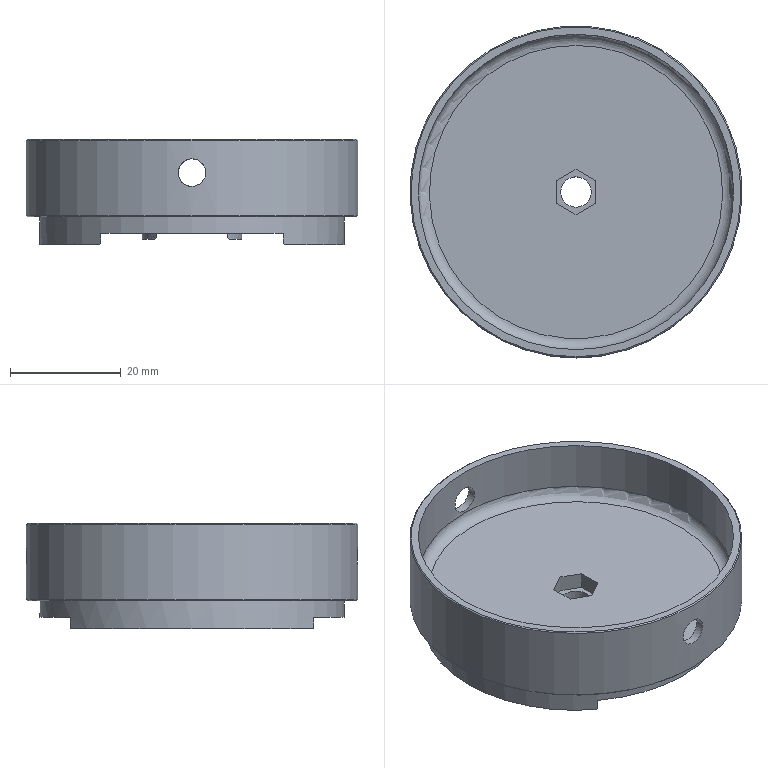Part | NX | 1 solid | 35 faces | box 60 x 60 x 19 mm | volume 19918 mm3 | plane 23 | cylinder 8 | cone 3 | torus 1 | commonest cylinder face diameters 5 x2 18 x2 5.5 x1 55 x1 57 x1 60 x1
STEP:
#1=CARTESIAN_POINT('',(0.,-2.75,-16.8));
#2=VERTEX_POINT('',#1);
#3=CARTESIAN_POINT('',(0.,0.,-16.8));
#4=DIRECTION('',(0.,0.,-1.));
#5=DIRECTION('',(0.,-1.,0.));
#6=AXIS2_PLACEMENT_3D('',#3,#4,#5);
#7=CIRCLE('',#6,2.75);
#8=EDGE_CURVE('',#2,#2,#7,.T.);
#9=ORIENTED_EDGE('',*,*,#8,.T.);
#10=EDGE_LOOP('',(#9));
#11=FACE_BOUND('',#10,.T.);
#12=CARTESIAN_POINT('',(0.,-2.75,-14.));
#13=VERTEX_POINT('',#12);
#14=CARTESIAN_POINT('',(0.,0.,-14.));
#15=DIRECTION('',(0.,0.,-1.));
#16=DIRECTION('',(0.,-1.,0.));
#17=AXIS2_PLACEMENT_3D('',#14,#15,#16);
#18=CIRCLE('',#17,2.75);
#19=EDGE_CURVE('',#13,#13,#18,.F.);
#20=ORIENTED_EDGE('',*,*,#19,.T.);
#21=EDGE_LOOP('',(#20));
#22=FACE_BOUND('',#21,.T.);
#23=CARTESIAN_POINT('',(0.,0.,0.));
#24=DIRECTION('',(0.,0.,-1.));
#25=DIRECTION('',(0.,-1.,0.));
#26=AXIS2_PLACEMENT_3D('',#23,#24,#25);
#27=CYLINDRICAL_SURFACE('',#26,2.75);
#28=ADVANCED_FACE('',(#11,#22),#27,.F.);
#29=CARTESIAN_POINT('',(-16.7,-21.849,-19.));
#30=VERTEX_POINT('',#29);
#31=CARTESIAN_POINT('',(-16.7,21.849,-19.));
#32=VERTEX_POINT('',#31);
#33=CARTESIAN_POINT('',(0.,0.,-19.));
#34=DIRECTION('',(0.,0.,-1.));
#35=DIRECTION('',(0.,-1.,0.));
#36=AXIS2_PLACEMENT_3D('',#33,#34,#35);
#37=CIRCLE('',#36,27.5);
#38=EDGE_CURVE('',#30,#32,#37,.T.);
#39=ORIENTED_EDGE('',*,*,#38,.T.);
#40=CARTESIAN_POINT('',(-16.7,-22.,-19.));
#41=DIRECTION('',(0.,-1.,0.));
#42=VECTOR('',#41,1000.);
#43=LINE('',#40,#42);
#44=EDGE_CURVE('',#32,#30,#43,.T.);
#45=ORIENTED_EDGE('',*,*,#44,.T.);
#46=EDGE_LOOP('',(#39,#45));
#47=FACE_BOUND('',#46,.T.);
#48=CARTESIAN_POINT('',(0.,0.,-19.));
#49=DIRECTION('',(0.,0.,-1.));
#50=DIRECTION('',(0.,-1.,0.));
#51=AXIS2_PLACEMENT_3D('',#48,#49,#50);
#52=PLANE('',#51);
#53=ADVANCED_FACE('',(#47),#52,.T.);
#54=CARTESIAN_POINT('',(0.,30.,-8.5));
#55=VERTEX_POINT('',#54);
#56=CARTESIAN_POINT('',(-1.961,29.948,-7.957));
#57=CARTESIAN_POINT('',(0.0004949,30.026,-8.771));
#58=CARTESIAN_POINT('',(1.959,29.948,-7.958));
#59=CARTESIAN_POINT('',(2.77,29.87,-6.002));
#60=CARTESIAN_POINT('',(1.96,29.948,-4.042));
#61=CARTESIAN_POINT('',(0.0004482,30.026,-3.23));
#62=CARTESIAN_POINT('',(-1.957,29.948,-4.039));
#63=CARTESIAN_POINT('',(-2.771,29.87,-5.997));
#64=CARTESIAN_POINT('',(-1.961,29.948,-7.957));
#65=CARTESIAN_POINT('',(0.0004949,30.026,-8.771));
#66=CARTESIAN_POINT('',(1.959,29.948,-7.958));
#67=B_SPLINE_CURVE_WITH_KNOTS('',3,(#56,#57,#58,#59,#60,#61,#62,#63,#64,#65,#66),.UNSPECIFIED.,.T.,.F.,(1,1,1,1,1,1,1,1,1,1,1,1,1,1,1),(-0.005864,-0.003909,-0.001955,0.,0.001955,0.003909,0.005864,0.007819,0.009773,0.01173,0.01368,0.01564,0.01759,0.01955,0.0215),.UNSPECIFIED.);
#68=EDGE_CURVE('',#55,#55,#67,.T.);
#69=ORIENTED_EDGE('',*,*,#68,.T.);
#70=EDGE_LOOP('',(#69));
#71=FACE_BOUND('',#70,.T.);
#72=CARTESIAN_POINT('',(-2.5,-29.896,-6.));
#73=VERTEX_POINT('',#72);
#74=CARTESIAN_POINT('',(-1.957,-29.948,-7.961));
#75=CARTESIAN_POINT('',(-2.771,-29.869,-6.));
#76=CARTESIAN_POINT('',(-1.958,-29.948,-4.041));
#77=CARTESIAN_POINT('',(-0.002118,-30.026,-3.23));
#78=CARTESIAN_POINT('',(1.958,-29.948,-4.04));
#79=CARTESIAN_POINT('',(2.77,-29.87,-6.));
#80=CARTESIAN_POINT('',(1.961,-29.948,-7.957));
#81=CARTESIAN_POINT('',(0.002777,-30.026,-8.771));
#82=CARTESIAN_POINT('',(-1.957,-29.948,-7.961));
#83=CARTESIAN_POINT('',(-2.771,-29.869,-6.));
#84=CARTESIAN_POINT('',(-1.958,-29.948,-4.041));
#85=B_SPLINE_CURVE_WITH_KNOTS('',3,(#74,#75,#76,#77,#78,#79,#80,#81,#82,#83,#84),.UNSPECIFIED.,.T.,.F.,(1,1,1,1,1,1,1,1,1,1,1,1,1,1,1),(-0.005864,-0.003909,-0.001955,0.,0.001955,0.003909,0.005864,0.007819,0.009773,0.01173,0.01368,0.01564,0.01759,0.01955,0.0215),.UNSPECIFIED.);
#86=EDGE_CURVE('',#73,#73,#85,.T.);
#87=ORIENTED_EDGE('',*,*,#86,.T.);
#88=EDGE_LOOP('',(#87));
#89=FACE_BOUND('',#88,.T.);
#90=CARTESIAN_POINT('',(0.,-30.,-13.8));
#91=VERTEX_POINT('',#90);
#92=CARTESIAN_POINT('',(0.,0.,-13.8));
#93=DIRECTION('',(0.,0.,-1.));
#94=DIRECTION('',(0.,-1.,0.));
#95=AXIS2_PLACEMENT_3D('',#92,#93,#94);
#96=CIRCLE('',#95,30.);
#97=EDGE_CURVE('',#91,#91,#96,.F.);
#98=ORIENTED_EDGE('',*,*,#97,.T.);
#99=EDGE_LOOP('',(#98));
#100=FACE_BOUND('',#99,.T.);
#101=CARTESIAN_POINT('',(0.,-30.,-0.2));
#102=VERTEX_POINT('',#101);
#103=CARTESIAN_POINT('',(0.,0.,-0.2));
#104=DIRECTION('',(0.,0.,-1.));
#105=DIRECTION('',(0.,-1.,0.));
#106=AXIS2_PLACEMENT_3D('',#103,#104,#105);
#107=CIRCLE('',#106,30.);
#108=EDGE_CURVE('',#102,#102,#107,.T.);
#109=ORIENTED_EDGE('',*,*,#108,.T.);
#110=EDGE_LOOP('',(#109));
#111=FACE_BOUND('',#110,.T.);
#112=CARTESIAN_POINT('',(0.,0.,-19.));
#113=DIRECTION('',(0.,0.,1.));
#114=DIRECTION('',(0.,1.,0.));
#115=AXIS2_PLACEMENT_3D('',#112,#113,#114);
#116=CYLINDRICAL_SURFACE('',#115,30.);
#117=ADVANCED_FACE('',(#71,#89,#100,#111),#116,.T.);
#118=CARTESIAN_POINT('',(0.,-29.8,0.));
#119=VERTEX_POINT('',#118);
#120=CARTESIAN_POINT('',(0.,0.,0.));
#121=DIRECTION('',(0.,0.,-1.));
#122=DIRECTION('',(0.,-1.,0.));
#123=AXIS2_PLACEMENT_3D('',#120,#121,#122);
#124=CIRCLE('',#123,29.8);
#125=EDGE_CURVE('',#119,#119,#124,.F.);
#126=ORIENTED_EDGE('',*,*,#125,.T.);
#127=EDGE_LOOP('',(#126));
#128=FACE_BOUND('',#127,.T.);
#129=CARTESIAN_POINT('',(0.,28.5,0.));
#130=VERTEX_POINT('',#129);
#131=CARTESIAN_POINT('',(0.,0.,0.));
#132=DIRECTION('',(0.,0.,1.));
#133=DIRECTION('',(0.,1.,0.));
#134=AXIS2_PLACEMENT_3D('',#131,#132,#133);
#135=CIRCLE('',#134,28.5);
#136=EDGE_CURVE('',#130,#130,#135,.T.);
#137=ORIENTED_EDGE('',*,*,#136,.F.);
#138=EDGE_LOOP('',(#137));
#139=FACE_BOUND('',#138,.T.);
#140=CARTESIAN_POINT('',(0.,0.,0.));
#141=DIRECTION('',(0.,0.,-1.));
#142=DIRECTION('',(0.,-1.,0.));
#143=AXIS2_PLACEMENT_3D('',#140,#141,#142);
#144=PLANE('',#143);
#145=ADVANCED_FACE('',(#128,#139),#144,.F.);
#146=CARTESIAN_POINT('',(0.,-29.8,-14.));
#147=VERTEX_POINT('',#146);
#148=CARTESIAN_POINT('',(0.,0.,-14.));
#149=DIRECTION('',(0.,0.,-1.));
#150=DIRECTION('',(0.,-1.,0.));
#151=AXIS2_PLACEMENT_3D('',#148,#149,#150);
#152=CIRCLE('',#151,29.8);
#153=EDGE_CURVE('',#147,#147,#152,.T.);
#154=ORIENTED_EDGE('',*,*,#153,.T.);
#155=EDGE_LOOP('',(#154));
#156=FACE_BOUND('',#155,.T.);
#157=CARTESIAN_POINT('',(0.,-27.5,-14.));
#158=VERTEX_POINT('',#157);
#159=CARTESIAN_POINT('',(0.,0.,-14.));
#160=DIRECTION('',(0.,0.,-1.));
#161=DIRECTION('',(0.,-1.,0.));
#162=AXIS2_PLACEMENT_3D('',#159,#160,#161);
#163=CIRCLE('',#162,27.5);
#164=EDGE_CURVE('',#158,#158,#163,.T.);
#165=ORIENTED_EDGE('',*,*,#164,.F.);
#166=EDGE_LOOP('',(#165));
#167=FACE_BOUND('',#166,.T.);
#168=CARTESIAN_POINT('',(0.,0.,-14.));
#169=DIRECTION('',(0.,0.,-1.));
#170=DIRECTION('',(0.,-1.,0.));
#171=AXIS2_PLACEMENT_3D('',#168,#169,#170);
#172=PLANE('',#171);
#173=ADVANCED_FACE('',(#156,#167),#172,.T.);
#174=CARTESIAN_POINT('',(-16.5,22.,-18.8));
#175=VERTEX_POINT('',#174);
#176=CARTESIAN_POINT('',(-16.5,22.,-17.));
#177=VERTEX_POINT('',#176);
#178=CARTESIAN_POINT('',(-16.5,22.,-17.));
#179=DIRECTION('',(0.,0.,-1.));
#180=VECTOR('',#179,1000.);
#181=LINE('',#178,#180);
#182=EDGE_CURVE('',#175,#177,#181,.F.);
#183=ORIENTED_EDGE('',*,*,#182,.F.);
#184=CARTESIAN_POINT('',(0.,0.,-2.3));
#185=DIRECTION('',(0.7071,0.,-0.7071));
#186=DIRECTION('',(-0.7071,0.,-0.7071));
#187=AXIS2_PLACEMENT_3D('',#184,#185,#186);
#188=ELLIPSE('',#187,38.891,27.5);
#189=EDGE_CURVE('',#175,#32,#188,.F.);
#190=ORIENTED_EDGE('',*,*,#189,.T.);
#191=ORIENTED_EDGE('',*,*,#38,.F.);
#192=CARTESIAN_POINT('',(-16.5,-22.,-18.8));
#193=VERTEX_POINT('',#192);
#194=CARTESIAN_POINT('',(0.,0.,-2.3));
#195=DIRECTION('',(0.7071,0.,-0.7071));
#196=DIRECTION('',(-0.7071,0.,-0.7071));
#197=AXIS2_PLACEMENT_3D('',#194,#195,#196);
#198=ELLIPSE('',#197,38.891,27.5);
#199=EDGE_CURVE('',#30,#193,#198,.F.);
#200=ORIENTED_EDGE('',*,*,#199,.T.);
#201=CARTESIAN_POINT('',(-16.5,-22.,-17.));
#202=VERTEX_POINT('',#201);
#203=CARTESIAN_POINT('',(-16.5,-22.,-17.));
#204=DIRECTION('',(0.,0.,-1.));
#205=VECTOR('',#204,1000.);
#206=LINE('',#203,#205);
#207=EDGE_CURVE('',#193,#202,#206,.F.);
#208=ORIENTED_EDGE('',*,*,#207,.T.);
#209=CARTESIAN_POINT('',(16.5,-22.,-17.));
#210=VERTEX_POINT('',#209);
#211=CARTESIAN_POINT('',(0.,0.,-17.));
#212=DIRECTION('',(0.,0.,-1.));
#213=DIRECTION('',(0.,-1.,0.));
#214=AXIS2_PLACEMENT_3D('',#211,#212,#213);
#215=CIRCLE('',#214,27.5);
#216=EDGE_CURVE('',#210,#202,#215,.T.);
#217=ORIENTED_EDGE('',*,*,#216,.F.);
#218=CARTESIAN_POINT('',(16.5,-22.,-18.8));
#219=VERTEX_POINT('',#218);
#220=CARTESIAN_POINT('',(16.5,-22.,-17.));
#221=DIRECTION('',(0.,0.,-1.));
#222=VECTOR('',#221,1000.);
#223=LINE('',#220,#222);
#224=EDGE_CURVE('',#219,#210,#223,.F.);
#225=ORIENTED_EDGE('',*,*,#224,.F.);
#226=CARTESIAN_POINT('',(16.7,-21.849,-19.));
#227=VERTEX_POINT('',#226);
#228=CARTESIAN_POINT('',(0.,0.,-2.3));
#229=DIRECTION('',(-0.7071,0.,-0.7071));
#230=DIRECTION('',(0.7071,0.,-0.7071));
#231=AXIS2_PLACEMENT_3D('',#228,#229,#230);
#232=ELLIPSE('',#231,38.891,27.5);
#233=EDGE_CURVE('',#219,#227,#232,.F.);
#234=ORIENTED_EDGE('',*,*,#233,.T.);
#235=CARTESIAN_POINT('',(16.7,21.849,-19.));
#236=VERTEX_POINT('',#235);
#237=CARTESIAN_POINT('',(0.,0.,-19.));
#238=DIRECTION('',(0.,0.,-1.));
#239=DIRECTION('',(0.,-1.,0.));
#240=AXIS2_PLACEMENT_3D('',#237,#238,#239);
#241=CIRCLE('',#240,27.5);
#242=EDGE_CURVE('',#236,#227,#241,.T.);
#243=ORIENTED_EDGE('',*,*,#242,.F.);
#244=CARTESIAN_POINT('',(16.5,22.,-18.8));
#245=VERTEX_POINT('',#244);
#246=CARTESIAN_POINT('',(0.,0.,-2.3));
#247=DIRECTION('',(-0.7071,0.,-0.7071));
#248=DIRECTION('',(0.7071,0.,-0.7071));
#249=AXIS2_PLACEMENT_3D('',#246,#247,#248);
#250=ELLIPSE('',#249,38.891,27.5);
#251=EDGE_CURVE('',#236,#245,#250,.F.);
#252=ORIENTED_EDGE('',*,*,#251,.T.);
#253=CARTESIAN_POINT('',(16.5,22.,-17.));
#254=VERTEX_POINT('',#253);
#255=CARTESIAN_POINT('',(16.5,22.,-17.));
#256=DIRECTION('',(0.,0.,-1.));
#257=VECTOR('',#256,1000.);
#258=LINE('',#255,#257);
#259=EDGE_CURVE('',#245,#254,#258,.F.);
#260=ORIENTED_EDGE('',*,*,#259,.T.);
#261=CARTESIAN_POINT('',(0.,0.,-17.));
#262=DIRECTION('',(0.,0.,-1.));
#263=DIRECTION('',(0.,-1.,0.));
#264=AXIS2_PLACEMENT_3D('',#261,#262,#263);
#265=CIRCLE('',#264,27.5);
#266=EDGE_CURVE('',#177,#254,#265,.T.);
#267=ORIENTED_EDGE('',*,*,#266,.F.);
#268=EDGE_LOOP('',(#183,#190,#191,#200,#208,#217,#225,#234,#243,#252,#260,#267));
#269=FACE_BOUND('',#268,.T.);
#270=ORIENTED_EDGE('',*,*,#164,.T.);
#271=EDGE_LOOP('',(#270));
#272=FACE_BOUND('',#271,.T.);
#273=CARTESIAN_POINT('',(0.,0.,-14.));
#274=DIRECTION('',(0.,0.,-1.));
#275=DIRECTION('',(0.,-1.,0.));
#276=AXIS2_PLACEMENT_3D('',#273,#274,#275);
#277=CYLINDRICAL_SURFACE('',#276,27.5);
#278=ADVANCED_FACE('',(#269,#272),#277,.T.);
#279=ORIENTED_EDGE('',*,*,#242,.T.);
#280=CARTESIAN_POINT('',(16.7,22.,-19.));
#281=DIRECTION('',(0.,1.,0.));
#282=VECTOR('',#281,1000.);
#283=LINE('',#280,#282);
#284=EDGE_CURVE('',#227,#236,#283,.T.);
#285=ORIENTED_EDGE('',*,*,#284,.T.);
#286=EDGE_LOOP('',(#279,#285));
#287=FACE_BOUND('',#286,.T.);
#288=CARTESIAN_POINT('',(0.,0.,-19.));
#289=DIRECTION('',(0.,0.,-1.));
#290=DIRECTION('',(0.,-1.,0.));
#291=AXIS2_PLACEMENT_3D('',#288,#289,#290);
#292=PLANE('',#291);
#293=ADVANCED_FACE('',(#287),#292,.T.);
#294=ORIENTED_EDGE('',*,*,#207,.F.);
#295=CARTESIAN_POINT('',(-16.5,22.,-18.8));
#296=DIRECTION('',(0.,1.,0.));
#297=VECTOR('',#296,1000.);
#298=LINE('',#295,#297);
#299=EDGE_CURVE('',#193,#175,#298,.T.);
#300=ORIENTED_EDGE('',*,*,#299,.T.);
#301=ORIENTED_EDGE('',*,*,#182,.T.);
#302=CARTESIAN_POINT('',(-16.5,22.,-17.));
#303=DIRECTION('',(0.,1.,0.));
#304=VECTOR('',#303,1000.);
#305=LINE('',#302,#304);
#306=EDGE_CURVE('',#202,#177,#305,.T.);
#307=ORIENTED_EDGE('',*,*,#306,.F.);
#308=EDGE_LOOP('',(#294,#300,#301,#307));
#309=FACE_BOUND('',#308,.T.);
#310=CARTESIAN_POINT('',(-16.5,22.,-17.));
#311=DIRECTION('',(-1.,0.,0.));
#312=DIRECTION('',(0.,1.,0.));
#313=AXIS2_PLACEMENT_3D('',#310,#311,#312);
#314=PLANE('',#313);
#315=ADVANCED_FACE('',(#309),#314,.F.);
#316=ORIENTED_EDGE('',*,*,#259,.F.);
#317=CARTESIAN_POINT('',(16.5,-22.,-18.8));
#318=DIRECTION('',(0.,-1.,0.));
#319=VECTOR('',#318,1000.);
#320=LINE('',#317,#319);
#321=EDGE_CURVE('',#245,#219,#320,.T.);
#322=ORIENTED_EDGE('',*,*,#321,.T.);
#323=ORIENTED_EDGE('',*,*,#224,.T.);
#324=CARTESIAN_POINT('',(16.5,22.,-17.));
#325=DIRECTION('',(0.,-1.,0.));
#326=VECTOR('',#325,1000.);
#327=LINE('',#324,#326);
#328=EDGE_CURVE('',#254,#210,#327,.T.);
#329=ORIENTED_EDGE('',*,*,#328,.F.);
#330=EDGE_LOOP('',(#316,#322,#323,#329));
#331=FACE_BOUND('',#330,.T.);
#332=CARTESIAN_POINT('',(16.5,22.,-17.));
#333=DIRECTION('',(1.,0.,0.));
#334=DIRECTION('',(0.,-1.,0.));
#335=AXIS2_PLACEMENT_3D('',#332,#333,#334);
#336=PLANE('',#335);
#337=ADVANCED_FACE('',(#331),#336,.F.);
#338=CARTESIAN_POINT('',(0.,-2.95,-17.));
#339=VERTEX_POINT('',#338);
#340=CARTESIAN_POINT('',(0.,0.,-17.));
#341=DIRECTION('',(0.,0.,-1.));
#342=DIRECTION('',(0.,-1.,0.));
#343=AXIS2_PLACEMENT_3D('',#340,#341,#342);
#344=CIRCLE('',#343,2.95);
#345=EDGE_CURVE('',#339,#339,#344,.F.);
#346=ORIENTED_EDGE('',*,*,#345,.T.);
#347=EDGE_LOOP('',(#346));
#348=FACE_BOUND('',#347,.T.);
#349=CARTESIAN_POINT('',(-6.5,6.225,-17.));
#350=VERTEX_POINT('',#349);
#351=CARTESIAN_POINT('',(-6.5,-6.225,-17.));
#352=VERTEX_POINT('',#351);
#353=CARTESIAN_POINT('',(-6.5,6.225,-17.));
#354=DIRECTION('',(0.,-1.,0.));
#355=VECTOR('',#354,1000.);
#356=LINE('',#353,#355);
#357=EDGE_CURVE('',#350,#352,#356,.T.);
#358=ORIENTED_EDGE('',*,*,#357,.F.);
#359=CARTESIAN_POINT('',(0.,0.,-17.));
#360=DIRECTION('',(0.,0.,-1.));
#361=DIRECTION('',(0.,-1.,0.));
#362=AXIS2_PLACEMENT_3D('',#359,#360,#361);
#363=CIRCLE('',#362,9.);
#364=EDGE_CURVE('',#352,#350,#363,.T.);
#365=ORIENTED_EDGE('',*,*,#364,.F.);
#366=EDGE_LOOP('',(#358,#365));
#367=FACE_BOUND('',#366,.T.);
#368=CARTESIAN_POINT('',(6.5,-6.225,-17.));
#369=VERTEX_POINT('',#368);
#370=CARTESIAN_POINT('',(6.5,6.225,-17.));
#371=VERTEX_POINT('',#370);
#372=CARTESIAN_POINT('',(6.5,6.225,-17.));
#373=DIRECTION('',(0.,1.,0.));
#374=VECTOR('',#373,1000.);
#375=LINE('',#372,#374);
#376=EDGE_CURVE('',#369,#371,#375,.T.);
#377=ORIENTED_EDGE('',*,*,#376,.F.);
#378=CARTESIAN_POINT('',(0.,0.,-17.));
#379=DIRECTION('',(0.,0.,-1.));
#380=DIRECTION('',(0.,-1.,0.));
#381=AXIS2_PLACEMENT_3D('',#378,#379,#380);
#382=CIRCLE('',#381,9.);
#383=EDGE_CURVE('',#371,#369,#382,.T.);
#384=ORIENTED_EDGE('',*,*,#383,.F.);
#385=EDGE_LOOP('',(#377,#384));
#386=FACE_BOUND('',#385,.T.);
#387=ORIENTED_EDGE('',*,*,#266,.T.);
#388=ORIENTED_EDGE('',*,*,#328,.T.);
#389=ORIENTED_EDGE('',*,*,#216,.T.);
#390=ORIENTED_EDGE('',*,*,#306,.T.);
#391=EDGE_LOOP('',(#387,#388,#389,#390));
#392=FACE_BOUND('',#391,.T.);
#393=CARTESIAN_POINT('',(0.,0.,-17.));
#394=DIRECTION('',(0.,0.,-1.));
#395=DIRECTION('',(0.,-1.,0.));
#396=AXIS2_PLACEMENT_3D('',#393,#394,#395);
#397=PLANE('',#396);
#398=ADVANCED_FACE('',(#348,#367,#386,#392),#397,.T.);
#399=CARTESIAN_POINT('',(6.7,6.009,-18.));
#400=VERTEX_POINT('',#399);
#401=CARTESIAN_POINT('',(6.7,-6.009,-18.));
#402=VERTEX_POINT('',#401);
#403=CARTESIAN_POINT('',(0.,0.,-18.));
#404=DIRECTION('',(0.,0.,1.));
#405=DIRECTION('',(0.,1.,0.));
#406=AXIS2_PLACEMENT_3D('',#403,#404,#405);
#407=CIRCLE('',#406,9.);
#408=EDGE_CURVE('',#400,#402,#407,.F.);
#409=ORIENTED_EDGE('',*,*,#408,.F.);
#410=CARTESIAN_POINT('',(6.5,6.225,-17.8));
#411=VERTEX_POINT('',#410);
#412=CARTESIAN_POINT('',(0.,0.,-11.3));
#413=DIRECTION('',(-0.7071,0.,-0.7071));
#414=DIRECTION('',(0.7071,0.,-0.7071));
#415=AXIS2_PLACEMENT_3D('',#412,#413,#414);
#416=ELLIPSE('',#415,12.728,9.);
#417=EDGE_CURVE('',#400,#411,#416,.F.);
#418=ORIENTED_EDGE('',*,*,#417,.T.);
#419=CARTESIAN_POINT('',(6.5,6.225,-17.));
#420=DIRECTION('',(0.,0.,-1.));
#421=VECTOR('',#420,1000.);
#422=LINE('',#419,#421);
#423=EDGE_CURVE('',#411,#371,#422,.F.);
#424=ORIENTED_EDGE('',*,*,#423,.T.);
#425=ORIENTED_EDGE('',*,*,#383,.T.);
#426=CARTESIAN_POINT('',(6.5,-6.225,-17.8));
#427=VERTEX_POINT('',#426);
#428=CARTESIAN_POINT('',(6.5,-6.225,-17.));
#429=DIRECTION('',(0.,0.,-1.));
#430=VECTOR('',#429,1000.);
#431=LINE('',#428,#430);
#432=EDGE_CURVE('',#427,#369,#431,.F.);
#433=ORIENTED_EDGE('',*,*,#432,.F.);
#434=CARTESIAN_POINT('',(0.,0.,-11.3));
#435=DIRECTION('',(-0.7071,0.,-0.7071));
#436=DIRECTION('',(0.7071,0.,-0.7071));
#437=AXIS2_PLACEMENT_3D('',#434,#435,#436);
#438=ELLIPSE('',#437,12.728,9.);
#439=EDGE_CURVE('',#427,#402,#438,.F.);
#440=ORIENTED_EDGE('',*,*,#439,.T.);
#441=EDGE_LOOP('',(#409,#418,#424,#425,#433,#440));
#442=FACE_BOUND('',#441,.T.);
#443=CARTESIAN_POINT('',(0.,0.,-17.));
#444=DIRECTION('',(0.,0.,-1.));
#445=DIRECTION('',(0.,-1.,0.));
#446=AXIS2_PLACEMENT_3D('',#443,#444,#445);
#447=CYLINDRICAL_SURFACE('',#446,9.);
#448=ADVANCED_FACE('',(#442),#447,.T.);
#449=ORIENTED_EDGE('',*,*,#423,.F.);
#450=CARTESIAN_POINT('',(6.5,-6.225,-17.8));
#451=DIRECTION('',(0.,-1.,0.));
#452=VECTOR('',#451,1000.);
#453=LINE('',#450,#452);
#454=EDGE_CURVE('',#411,#427,#453,.T.);
#455=ORIENTED_EDGE('',*,*,#454,.T.);
#456=ORIENTED_EDGE('',*,*,#432,.T.);
#457=ORIENTED_EDGE('',*,*,#376,.T.);
#458=EDGE_LOOP('',(#449,#455,#456,#457));
#459=FACE_BOUND('',#458,.T.);
#460=CARTESIAN_POINT('',(6.5,6.225,-17.));
#461=DIRECTION('',(-1.,0.,0.));
#462=DIRECTION('',(0.,1.,0.));
#463=AXIS2_PLACEMENT_3D('',#460,#461,#462);
#464=PLANE('',#463);
#465=ADVANCED_FACE('',(#459),#464,.T.);
#466=CARTESIAN_POINT('',(-6.7,-6.009,-18.));
#467=VERTEX_POINT('',#466);
#468=CARTESIAN_POINT('',(-6.7,6.009,-18.));
#469=VERTEX_POINT('',#468);
#470=CARTESIAN_POINT('',(0.,0.,-18.));
#471=DIRECTION('',(0.,0.,1.));
#472=DIRECTION('',(0.,1.,0.));
#473=AXIS2_PLACEMENT_3D('',#470,#471,#472);
#474=CIRCLE('',#473,9.);
#475=EDGE_CURVE('',#467,#469,#474,.F.);
#476=ORIENTED_EDGE('',*,*,#475,.F.);
#477=CARTESIAN_POINT('',(-6.5,-6.225,-17.8));
#478=VERTEX_POINT('',#477);
#479=CARTESIAN_POINT('',(0.,0.,-11.3));
#480=DIRECTION('',(0.7071,0.,-0.7071));
#481=DIRECTION('',(-0.7071,0.,-0.7071));
#482=AXIS2_PLACEMENT_3D('',#479,#480,#481);
#483=ELLIPSE('',#482,12.728,9.);
#484=EDGE_CURVE('',#467,#478,#483,.F.);
#485=ORIENTED_EDGE('',*,*,#484,.T.);
#486=CARTESIAN_POINT('',(-6.5,-6.225,-17.));
#487=DIRECTION('',(0.,0.,-1.));
#488=VECTOR('',#487,1000.);
#489=LINE('',#486,#488);
#490=EDGE_CURVE('',#478,#352,#489,.F.);
#491=ORIENTED_EDGE('',*,*,#490,.T.);
#492=ORIENTED_EDGE('',*,*,#364,.T.);
#493=CARTESIAN_POINT('',(-6.5,6.225,-17.8));
#494=VERTEX_POINT('',#493);
#495=CARTESIAN_POINT('',(-6.5,6.225,-17.));
#496=DIRECTION('',(0.,0.,-1.));
#497=VECTOR('',#496,1000.);
#498=LINE('',#495,#497);
#499=EDGE_CURVE('',#494,#350,#498,.F.);
#500=ORIENTED_EDGE('',*,*,#499,.F.);
#501=CARTESIAN_POINT('',(0.,0.,-11.3));
#502=DIRECTION('',(0.7071,0.,-0.7071));
#503=DIRECTION('',(-0.7071,0.,-0.7071));
#504=AXIS2_PLACEMENT_3D('',#501,#502,#503);
#505=ELLIPSE('',#504,12.728,9.);
#506=EDGE_CURVE('',#494,#469,#505,.F.);
#507=ORIENTED_EDGE('',*,*,#506,.T.);
#508=EDGE_LOOP('',(#476,#485,#491,#492,#500,#507));
#509=FACE_BOUND('',#508,.T.);
#510=CARTESIAN_POINT('',(0.,0.,-17.));
#511=DIRECTION('',(0.,0.,-1.));
#512=DIRECTION('',(0.,-1.,0.));
#513=AXIS2_PLACEMENT_3D('',#510,#511,#512);
#514=CYLINDRICAL_SURFACE('',#513,9.);
#515=ADVANCED_FACE('',(#509),#514,.T.);
#516=ORIENTED_EDGE('',*,*,#490,.F.);
#517=CARTESIAN_POINT('',(-6.5,6.225,-17.8));
#518=DIRECTION('',(0.,1.,0.));
#519=VECTOR('',#518,1000.);
#520=LINE('',#517,#519);
#521=EDGE_CURVE('',#478,#494,#520,.T.);
#522=ORIENTED_EDGE('',*,*,#521,.T.);
#523=ORIENTED_EDGE('',*,*,#499,.T.);
#524=ORIENTED_EDGE('',*,*,#357,.T.);
#525=EDGE_LOOP('',(#516,#522,#523,#524));
#526=FACE_BOUND('',#525,.T.);
#527=CARTESIAN_POINT('',(-6.5,6.225,-17.));
#528=DIRECTION('',(1.,0.,0.));
#529=DIRECTION('',(0.,-1.,0.));
#530=AXIS2_PLACEMENT_3D('',#527,#528,#529);
#531=PLANE('',#530);
#532=ADVANCED_FACE('',(#526),#531,.T.);
#533=CARTESIAN_POINT('',(0.,26.5,-11.));
#534=VERTEX_POINT('',#533);
#535=CARTESIAN_POINT('',(0.,0.,-11.));
#536=DIRECTION('',(0.,0.,1.));
#537=DIRECTION('',(0.,1.,0.));
#538=AXIS2_PLACEMENT_3D('',#535,#536,#537);
#539=CIRCLE('',#538,26.5);
#540=EDGE_CURVE('',#534,#534,#539,.T.);
#541=ORIENTED_EDGE('',*,*,#540,.T.);
#542=EDGE_LOOP('',(#541));
#543=FACE_BOUND('',#542,.T.);
#544=CARTESIAN_POINT('',(0.,-4.099,-11.));
#545=VERTEX_POINT('',#544);
#546=CARTESIAN_POINT('',(3.55,-2.05,-11.));
#547=VERTEX_POINT('',#546);
#548=CARTESIAN_POINT('',(0.,-4.099,-11.));
#549=DIRECTION('',(0.866,0.5,0.));
#550=VECTOR('',#549,1000.);
#551=LINE('',#548,#550);
#552=EDGE_CURVE('',#545,#547,#551,.T.);
#553=ORIENTED_EDGE('',*,*,#552,.F.);
#554=CARTESIAN_POINT('',(-3.55,-2.05,-11.));
#555=VERTEX_POINT('',#554);
#556=CARTESIAN_POINT('',(-3.55,-2.05,-11.));
#557=DIRECTION('',(0.866,-0.5,0.));
#558=VECTOR('',#557,1000.);
#559=LINE('',#556,#558);
#560=EDGE_CURVE('',#555,#545,#559,.T.);
#561=ORIENTED_EDGE('',*,*,#560,.F.);
#562=CARTESIAN_POINT('',(-3.55,2.05,-11.));
#563=VERTEX_POINT('',#562);
#564=CARTESIAN_POINT('',(-3.55,2.05,-11.));
#565=DIRECTION('',(0.,-1.,0.));
#566=VECTOR('',#565,1000.);
#567=LINE('',#564,#566);
#568=EDGE_CURVE('',#563,#555,#567,.T.);
#569=ORIENTED_EDGE('',*,*,#568,.F.);
#570=CARTESIAN_POINT('',(0.,4.099,-11.));
#571=VERTEX_POINT('',#570);
#572=CARTESIAN_POINT('',(0.,4.099,-11.));
#573=DIRECTION('',(-0.866,-0.5,0.));
#574=VECTOR('',#573,1000.);
#575=LINE('',#572,#574);
#576=EDGE_CURVE('',#571,#563,#575,.T.);
#577=ORIENTED_EDGE('',*,*,#576,.F.);
#578=CARTESIAN_POINT('',(3.55,2.05,-11.));
#579=VERTEX_POINT('',#578);
#580=CARTESIAN_POINT('',(3.55,2.05,-11.));
#581=DIRECTION('',(-0.866,0.5,0.));
#582=VECTOR('',#581,1000.);
#583=LINE('',#580,#582);
#584=EDGE_CURVE('',#579,#571,#583,.T.);
#585=ORIENTED_EDGE('',*,*,#584,.F.);
#586=CARTESIAN_POINT('',(3.55,-2.05,-11.));
#587=DIRECTION('',(0.,1.,0.));
#588=VECTOR('',#587,1000.);
#589=LINE('',#586,#588);
#590=EDGE_CURVE('',#547,#579,#589,.T.);
#591=ORIENTED_EDGE('',*,*,#590,.F.);
#592=EDGE_LOOP('',(#553,#561,#569,#577,#585,#591));
#593=FACE_BOUND('',#592,.T.);
#594=CARTESIAN_POINT('',(0.,0.,-11.));
#595=DIRECTION('',(0.,0.,1.));
#596=DIRECTION('',(0.,1.,0.));
#597=AXIS2_PLACEMENT_3D('',#594,#595,#596);
#598=PLANE('',#597);
#599=ADVANCED_FACE('',(#543,#593),#598,.T.);
#600=CARTESIAN_POINT('',(0.,28.5,-8.5));
#601=VERTEX_POINT('',#600);
#602=CARTESIAN_POINT('',(1.961,28.445,-7.957));
#603=CARTESIAN_POINT('',(-0.0004939,28.527,-8.771));
#604=CARTESIAN_POINT('',(-1.959,28.445,-7.958));
#605=CARTESIAN_POINT('',(-2.77,28.363,-6.002));
#606=CARTESIAN_POINT('',(-1.96,28.445,-4.042));
#607=CARTESIAN_POINT('',(-0.0004583,28.527,-3.23));
#608=CARTESIAN_POINT('',(1.957,28.445,-4.039));
#609=CARTESIAN_POINT('',(2.771,28.363,-5.997));
#610=CARTESIAN_POINT('',(1.961,28.445,-7.957));
#611=CARTESIAN_POINT('',(-0.0004939,28.527,-8.771));
#612=CARTESIAN_POINT('',(-1.959,28.445,-7.958));
#613=B_SPLINE_CURVE_WITH_KNOTS('',3,(#602,#603,#604,#605,#606,#607,#608,#609,#610,#611,#612),.UNSPECIFIED.,.T.,.F.,(1,1,1,1,1,1,1,1,1,1,1,1,1,1,1),(-0.005864,-0.003909,-0.001955,0.,0.001955,0.003909,0.005864,0.007819,0.009774,0.01173,0.01368,0.01564,0.01759,0.01955,0.0215),.UNSPECIFIED.);
#614=EDGE_CURVE('',#601,#601,#613,.T.);
#615=ORIENTED_EDGE('',*,*,#614,.T.);
#616=EDGE_LOOP('',(#615));
#617=FACE_BOUND('',#616,.T.);
#618=CARTESIAN_POINT('',(-2.5,-28.39,-6.));
#619=VERTEX_POINT('',#618);
#620=CARTESIAN_POINT('',(-1.957,-28.445,-4.039));
#621=CARTESIAN_POINT('',(-2.771,-28.363,-6.));
#622=CARTESIAN_POINT('',(-1.958,-28.445,-7.959));
#623=CARTESIAN_POINT('',(-0.002129,-28.527,-8.77));
#624=CARTESIAN_POINT('',(1.958,-28.445,-7.96));
#625=CARTESIAN_POINT('',(2.77,-28.363,-6.));
#626=CARTESIAN_POINT('',(1.961,-28.445,-4.043));
#627=CARTESIAN_POINT('',(0.002754,-28.527,-3.229));
#628=CARTESIAN_POINT('',(-1.957,-28.445,-4.039));
#629=CARTESIAN_POINT('',(-2.771,-28.363,-6.));
#630=CARTESIAN_POINT('',(-1.958,-28.445,-7.959));
#631=B_SPLINE_CURVE_WITH_KNOTS('',3,(#620,#621,#622,#623,#624,#625,#626,#627,#628,#629,#630),.UNSPECIFIED.,.T.,.F.,(1,1,1,1,1,1,1,1,1,1,1,1,1,1,1),(-0.005864,-0.003909,-0.001955,0.,0.001955,0.003909,0.005864,0.007819,0.009774,0.01173,0.01368,0.01564,0.01759,0.01955,0.0215),.UNSPECIFIED.);
#632=EDGE_CURVE('',#619,#619,#631,.T.);
#633=ORIENTED_EDGE('',*,*,#632,.T.);
#634=EDGE_LOOP('',(#633));
#635=FACE_BOUND('',#634,.T.);
#636=CARTESIAN_POINT('',(0.,28.5,-9.));
#637=VERTEX_POINT('',#636);
#638=CARTESIAN_POINT('',(0.,0.,-9.));
#639=DIRECTION('',(0.,0.,1.));
#640=DIRECTION('',(0.,1.,0.));
#641=AXIS2_PLACEMENT_3D('',#638,#639,#640);
#642=CIRCLE('',#641,28.5);
#643=EDGE_CURVE('',#637,#637,#642,.F.);
#644=ORIENTED_EDGE('',*,*,#643,.T.);
#645=EDGE_LOOP('',(#644));
#646=FACE_BOUND('',#645,.T.);
#647=ORIENTED_EDGE('',*,*,#136,.T.);
#648=EDGE_LOOP('',(#647));
#649=FACE_BOUND('',#648,.T.);
#650=CARTESIAN_POINT('',(0.,0.,-11.));
#651=DIRECTION('',(0.,0.,1.));
#652=DIRECTION('',(0.,1.,0.));
#653=AXIS2_PLACEMENT_3D('',#650,#651,#652);
#654=CYLINDRICAL_SURFACE('',#653,28.5);
#655=ADVANCED_FACE('',(#617,#635,#646,#649),#654,.F.);
#656=CARTESIAN_POINT('',(-3.55,-2.05,-14.));
#657=VERTEX_POINT('',#656);
#658=CARTESIAN_POINT('',(0.,-4.099,-14.));
#659=VERTEX_POINT('',#658);
#660=CARTESIAN_POINT('',(-3.55,-2.05,-14.));
#661=DIRECTION('',(0.866,-0.5,0.));
#662=VECTOR('',#661,1000.);
#663=LINE('',#660,#662);
#664=EDGE_CURVE('',#657,#659,#663,.T.);
#665=ORIENTED_EDGE('',*,*,#664,.T.);
#666=CARTESIAN_POINT('',(3.55,-2.05,-14.));
#667=VERTEX_POINT('',#666);
#668=CARTESIAN_POINT('',(0.,-4.099,-14.));
#669=DIRECTION('',(0.866,0.5,0.));
#670=VECTOR('',#669,1000.);
#671=LINE('',#668,#670);
#672=EDGE_CURVE('',#659,#667,#671,.T.);
#673=ORIENTED_EDGE('',*,*,#672,.T.);
#674=CARTESIAN_POINT('',(3.55,2.05,-14.));
#675=VERTEX_POINT('',#674);
#676=CARTESIAN_POINT('',(3.55,-2.05,-14.));
#677=DIRECTION('',(0.,1.,0.));
#678=VECTOR('',#677,1000.);
#679=LINE('',#676,#678);
#680=EDGE_CURVE('',#667,#675,#679,.T.);
#681=ORIENTED_EDGE('',*,*,#680,.T.);
#682=CARTESIAN_POINT('',(0.,4.099,-14.));
#683=VERTEX_POINT('',#682);
#684=CARTESIAN_POINT('',(3.55,2.05,-14.));
#685=DIRECTION('',(-0.866,0.5,0.));
#686=VECTOR('',#685,1000.);
#687=LINE('',#684,#686);
#688=EDGE_CURVE('',#675,#683,#687,.T.);
#689=ORIENTED_EDGE('',*,*,#688,.T.);
#690=CARTESIAN_POINT('',(-3.55,2.05,-14.));
#691=VERTEX_POINT('',#690);
#692=CARTESIAN_POINT('',(0.,4.099,-14.));
#693=DIRECTION('',(-0.866,-0.5,0.));
#694=VECTOR('',#693,1000.);
#695=LINE('',#692,#694);
#696=EDGE_CURVE('',#683,#691,#695,.T.);
#697=ORIENTED_EDGE('',*,*,#696,.T.);
#698=CARTESIAN_POINT('',(-3.55,2.05,-14.));
#699=DIRECTION('',(0.,-1.,0.));
#700=VECTOR('',#699,1000.);
#701=LINE('',#698,#700);
#702=EDGE_CURVE('',#691,#657,#701,.T.);
#703=ORIENTED_EDGE('',*,*,#702,.T.);
#704=EDGE_LOOP('',(#665,#673,#681,#689,#697,#703));
#705=FACE_BOUND('',#704,.T.);
#706=ORIENTED_EDGE('',*,*,#19,.F.);
#707=EDGE_LOOP('',(#706));
#708=FACE_BOUND('',#707,.T.);
#709=CARTESIAN_POINT('',(0.,0.,-14.));
#710=DIRECTION('',(0.,0.,-1.));
#711=DIRECTION('',(0.,-1.,0.));
#712=AXIS2_PLACEMENT_3D('',#709,#710,#711);
#713=PLANE('',#712);
#714=ADVANCED_FACE('',(#705,#708),#713,.F.);
#715=CARTESIAN_POINT('',(0.,-4.099,-27.845));
#716=DIRECTION('',(0.,0.,1.));
#717=VECTOR('',#716,1000.);
#718=LINE('',#715,#717);
#719=EDGE_CURVE('',#659,#545,#718,.T.);
#720=ORIENTED_EDGE('',*,*,#719,.T.);
#721=ORIENTED_EDGE('',*,*,#552,.T.);
#722=CARTESIAN_POINT('',(3.55,-2.05,-27.845));
#723=DIRECTION('',(0.,0.,1.));
#724=VECTOR('',#723,1000.);
#725=LINE('',#722,#724);
#726=EDGE_CURVE('',#667,#547,#725,.T.);
#727=ORIENTED_EDGE('',*,*,#726,.F.);
#728=ORIENTED_EDGE('',*,*,#672,.F.);
#729=EDGE_LOOP('',(#720,#721,#727,#728));
#730=FACE_BOUND('',#729,.T.);
#731=CARTESIAN_POINT('',(0.,-4.099,-27.845));
#732=DIRECTION('',(0.5,-0.866,0.));
#733=DIRECTION('',(-0.866,-0.5,0.));
#734=AXIS2_PLACEMENT_3D('',#731,#732,#733);
#735=PLANE('',#734);
#736=ADVANCED_FACE('',(#730),#735,.F.);
#737=ORIENTED_EDGE('',*,*,#726,.T.);
#738=ORIENTED_EDGE('',*,*,#590,.T.);
#739=CARTESIAN_POINT('',(3.55,2.05,-27.845));
#740=DIRECTION('',(0.,0.,1.));
#741=VECTOR('',#740,1000.);
#742=LINE('',#739,#741);
#743=EDGE_CURVE('',#675,#579,#742,.T.);
#744=ORIENTED_EDGE('',*,*,#743,.F.);
#745=ORIENTED_EDGE('',*,*,#680,.F.);
#746=EDGE_LOOP('',(#737,#738,#744,#745));
#747=FACE_BOUND('',#746,.T.);
#748=CARTESIAN_POINT('',(3.55,-2.05,-27.845));
#749=DIRECTION('',(1.,0.,0.));
#750=DIRECTION('',(0.,-1.,0.));
#751=AXIS2_PLACEMENT_3D('',#748,#749,#750);
#752=PLANE('',#751);
#753=ADVANCED_FACE('',(#747),#752,.F.);
#754=ORIENTED_EDGE('',*,*,#743,.T.);
#755=ORIENTED_EDGE('',*,*,#584,.T.);
#756=CARTESIAN_POINT('',(0.,4.099,-27.845));
#757=DIRECTION('',(0.,0.,1.));
#758=VECTOR('',#757,1000.);
#759=LINE('',#756,#758);
#760=EDGE_CURVE('',#683,#571,#759,.T.);
#761=ORIENTED_EDGE('',*,*,#760,.F.);
#762=ORIENTED_EDGE('',*,*,#688,.F.);
#763=EDGE_LOOP('',(#754,#755,#761,#762));
#764=FACE_BOUND('',#763,.T.);
#765=CARTESIAN_POINT('',(3.55,2.05,-27.845));
#766=DIRECTION('',(0.5,0.866,0.));
#767=DIRECTION('',(0.866,-0.5,0.));
#768=AXIS2_PLACEMENT_3D('',#765,#766,#767);
#769=PLANE('',#768);
#770=ADVANCED_FACE('',(#764),#769,.F.);
#771=ORIENTED_EDGE('',*,*,#760,.T.);
#772=ORIENTED_EDGE('',*,*,#576,.T.);
#773=CARTESIAN_POINT('',(-3.55,2.05,-27.845));
#774=DIRECTION('',(0.,0.,1.));
#775=VECTOR('',#774,1000.);
#776=LINE('',#773,#775);
#777=EDGE_CURVE('',#691,#563,#776,.T.);
#778=ORIENTED_EDGE('',*,*,#777,.F.);
#779=ORIENTED_EDGE('',*,*,#696,.F.);
#780=EDGE_LOOP('',(#771,#772,#778,#779));
#781=FACE_BOUND('',#780,.T.);
#782=CARTESIAN_POINT('',(0.,4.099,-27.845));
#783=DIRECTION('',(-0.5,0.866,0.));
#784=DIRECTION('',(0.866,0.5,0.));
#785=AXIS2_PLACEMENT_3D('',#782,#783,#784);
#786=PLANE('',#785);
#787=ADVANCED_FACE('',(#781),#786,.F.);
#788=ORIENTED_EDGE('',*,*,#777,.T.);
#789=ORIENTED_EDGE('',*,*,#568,.T.);
#790=CARTESIAN_POINT('',(-3.55,-2.05,-27.845));
#791=DIRECTION('',(0.,0.,1.));
#792=VECTOR('',#791,1000.);
#793=LINE('',#790,#792);
#794=EDGE_CURVE('',#657,#555,#793,.T.);
#795=ORIENTED_EDGE('',*,*,#794,.F.);
#796=ORIENTED_EDGE('',*,*,#702,.F.);
#797=EDGE_LOOP('',(#788,#789,#795,#796));
#798=FACE_BOUND('',#797,.T.);
#799=CARTESIAN_POINT('',(-3.55,2.05,-27.845));
#800=DIRECTION('',(-1.,0.,0.));
#801=DIRECTION('',(0.,1.,0.));
#802=AXIS2_PLACEMENT_3D('',#799,#800,#801);
#803=PLANE('',#802);
#804=ADVANCED_FACE('',(#798),#803,.F.);
#805=ORIENTED_EDGE('',*,*,#794,.T.);
#806=ORIENTED_EDGE('',*,*,#560,.T.);
#807=ORIENTED_EDGE('',*,*,#719,.F.);
#808=ORIENTED_EDGE('',*,*,#664,.F.);
#809=EDGE_LOOP('',(#805,#806,#807,#808));
#810=FACE_BOUND('',#809,.T.);
#811=CARTESIAN_POINT('',(-3.55,-2.05,-27.845));
#812=DIRECTION('',(-0.5,-0.866,0.));
#813=DIRECTION('',(-0.866,0.5,0.));
#814=AXIS2_PLACEMENT_3D('',#811,#812,#813);
#815=PLANE('',#814);
#816=ADVANCED_FACE('',(#810),#815,.F.);
#817=ORIENTED_EDGE('',*,*,#475,.T.);
#818=CARTESIAN_POINT('',(-6.7,-6.225,-18.));
#819=DIRECTION('',(0.,-1.,0.));
#820=VECTOR('',#819,1000.);
#821=LINE('',#818,#820);
#822=EDGE_CURVE('',#469,#467,#821,.T.);
#823=ORIENTED_EDGE('',*,*,#822,.T.);
#824=EDGE_LOOP('',(#817,#823));
#825=FACE_BOUND('',#824,.T.);
#826=CARTESIAN_POINT('',(9.,30.,-18.));
#827=DIRECTION('',(0.,0.,1.));
#828=DIRECTION('',(0.,1.,0.));
#829=AXIS2_PLACEMENT_3D('',#826,#827,#828);
#830=PLANE('',#829);
#831=ADVANCED_FACE('',(#825),#830,.F.);
#832=ORIENTED_EDGE('',*,*,#408,.T.);
#833=CARTESIAN_POINT('',(6.7,6.225,-18.));
#834=DIRECTION('',(0.,1.,0.));
#835=VECTOR('',#834,1000.);
#836=LINE('',#833,#835);
#837=EDGE_CURVE('',#402,#400,#836,.T.);
#838=ORIENTED_EDGE('',*,*,#837,.T.);
#839=EDGE_LOOP('',(#832,#838));
#840=FACE_BOUND('',#839,.T.);
#841=CARTESIAN_POINT('',(9.,30.,-18.));
#842=DIRECTION('',(0.,0.,1.));
#843=DIRECTION('',(0.,1.,0.));
#844=AXIS2_PLACEMENT_3D('',#841,#842,#843);
#845=PLANE('',#844);
#846=ADVANCED_FACE('',(#840),#845,.F.);
#847=ORIENTED_EDGE('',*,*,#643,.F.);
#848=EDGE_LOOP('',(#847));
#849=FACE_BOUND('',#848,.T.);
#850=ORIENTED_EDGE('',*,*,#540,.F.);
#851=EDGE_LOOP('',(#850));
#852=FACE_BOUND('',#851,.T.);
#853=CARTESIAN_POINT('',(0.,0.,-9.));
#854=DIRECTION('',(0.,0.,1.));
#855=DIRECTION('',(0.,1.,0.));
#856=AXIS2_PLACEMENT_3D('',#853,#854,#855);
#857=TOROIDAL_SURFACE('',#856,26.5,2.);
#858=ADVANCED_FACE('',(#849,#852),#857,.F.);
#859=ORIENTED_EDGE('',*,*,#97,.F.);
#860=EDGE_LOOP('',(#859));
#861=FACE_BOUND('',#860,.T.);
#862=ORIENTED_EDGE('',*,*,#153,.F.);
#863=EDGE_LOOP('',(#862));
#864=FACE_BOUND('',#863,.T.);
#865=CARTESIAN_POINT('',(0.,0.,-14.));
#866=DIRECTION('',(0.,0.,1.));
#867=DIRECTION('',(0.,1.,0.));
#868=AXIS2_PLACEMENT_3D('',#865,#866,#867);
#869=CONICAL_SURFACE('',#868,29.8,0.7854);
#870=ADVANCED_FACE('',(#861,#864),#869,.T.);
#871=ORIENTED_EDGE('',*,*,#125,.F.);
#872=EDGE_LOOP('',(#871));
#873=FACE_BOUND('',#872,.T.);
#874=ORIENTED_EDGE('',*,*,#108,.F.);
#875=EDGE_LOOP('',(#874));
#876=FACE_BOUND('',#875,.T.);
#877=CARTESIAN_POINT('',(0.,0.,-0.2));
#878=DIRECTION('',(0.,0.,-1.));
#879=DIRECTION('',(0.,-1.,0.));
#880=AXIS2_PLACEMENT_3D('',#877,#878,#879);
#881=CONICAL_SURFACE('',#880,30.,0.7854);
#882=ADVANCED_FACE('',(#873,#876),#881,.T.);
#883=ORIENTED_EDGE('',*,*,#345,.F.);
#884=EDGE_LOOP('',(#883));
#885=FACE_BOUND('',#884,.T.);
#886=ORIENTED_EDGE('',*,*,#8,.F.);
#887=EDGE_LOOP('',(#886));
#888=FACE_BOUND('',#887,.T.);
#889=CARTESIAN_POINT('',(0.,0.,-16.8));
#890=DIRECTION('',(0.,0.,-1.));
#891=DIRECTION('',(0.,-1.,0.));
#892=AXIS2_PLACEMENT_3D('',#889,#890,#891);
#893=CONICAL_SURFACE('',#892,2.75,0.7854);
#894=ADVANCED_FACE('',(#885,#888),#893,.F.);
#895=ORIENTED_EDGE('',*,*,#439,.F.);
#896=ORIENTED_EDGE('',*,*,#454,.F.);
#897=ORIENTED_EDGE('',*,*,#417,.F.);
#898=ORIENTED_EDGE('',*,*,#837,.F.);
#899=EDGE_LOOP('',(#895,#896,#897,#898));
#900=FACE_BOUND('',#899,.T.);
#901=CARTESIAN_POINT('',(6.7,30.,-18.));
#902=DIRECTION('',(-0.7071,0.,-0.7071));
#903=DIRECTION('',(0.,-1.,0.));
#904=AXIS2_PLACEMENT_3D('',#901,#902,#903);
#905=PLANE('',#904);
#906=ADVANCED_FACE('',(#900),#905,.T.);
#907=ORIENTED_EDGE('',*,*,#506,.F.);
#908=ORIENTED_EDGE('',*,*,#521,.F.);
#909=ORIENTED_EDGE('',*,*,#484,.F.);
#910=ORIENTED_EDGE('',*,*,#822,.F.);
#911=EDGE_LOOP('',(#907,#908,#909,#910));
#912=FACE_BOUND('',#911,.T.);
#913=CARTESIAN_POINT('',(-6.7,30.,-18.));
#914=DIRECTION('',(0.7071,0.,-0.7071));
#915=DIRECTION('',(0.,1.,0.));
#916=AXIS2_PLACEMENT_3D('',#913,#914,#915);
#917=PLANE('',#916);
#918=ADVANCED_FACE('',(#912),#917,.T.);
#919=ORIENTED_EDGE('',*,*,#199,.F.);
#920=ORIENTED_EDGE('',*,*,#44,.F.);
#921=ORIENTED_EDGE('',*,*,#189,.F.);
#922=ORIENTED_EDGE('',*,*,#299,.F.);
#923=EDGE_LOOP('',(#919,#920,#921,#922));
#924=FACE_BOUND('',#923,.T.);
#925=CARTESIAN_POINT('',(-16.5,22.,-18.8));
#926=DIRECTION('',(0.7071,0.,-0.7071));
#927=DIRECTION('',(0.,-1.,0.));
#928=AXIS2_PLACEMENT_3D('',#925,#926,#927);
#929=PLANE('',#928);
#930=ADVANCED_FACE('',(#924),#929,.T.);
#931=ORIENTED_EDGE('',*,*,#251,.F.);
#932=ORIENTED_EDGE('',*,*,#284,.F.);
#933=ORIENTED_EDGE('',*,*,#233,.F.);
#934=ORIENTED_EDGE('',*,*,#321,.F.);
#935=EDGE_LOOP('',(#931,#932,#933,#934));
#936=FACE_BOUND('',#935,.T.);
#937=CARTESIAN_POINT('',(16.5,22.,-18.8));
#938=DIRECTION('',(-0.7071,0.,-0.7071));
#939=DIRECTION('',(0.,1.,0.));
#940=AXIS2_PLACEMENT_3D('',#937,#938,#939);
#941=PLANE('',#940);
#942=ADVANCED_FACE('',(#936),#941,.T.);
#943=ORIENTED_EDGE('',*,*,#632,.F.);
#944=EDGE_LOOP('',(#943));
#945=FACE_BOUND('',#944,.T.);
#946=ORIENTED_EDGE('',*,*,#86,.F.);
#947=EDGE_LOOP('',(#946));
#948=FACE_BOUND('',#947,.T.);
#949=CARTESIAN_POINT('',(0.,30.,-6.));
#950=DIRECTION('',(0.,-1.,0.));
#951=DIRECTION('',(-1.,0.,0.));
#952=AXIS2_PLACEMENT_3D('',#949,#950,#951);
#953=CYLINDRICAL_SURFACE('',#952,2.5);
#954=ADVANCED_FACE('',(#945,#948),#953,.F.);
#955=ORIENTED_EDGE('',*,*,#614,.F.);
#956=EDGE_LOOP('',(#955));
#957=FACE_BOUND('',#956,.T.);
#958=ORIENTED_EDGE('',*,*,#68,.F.);
#959=EDGE_LOOP('',(#958));
#960=FACE_BOUND('',#959,.T.);
#961=CARTESIAN_POINT('',(0.,30.,-6.));
#962=DIRECTION('',(0.,-1.,0.));
#963=DIRECTION('',(-1.,0.,0.));
#964=AXIS2_PLACEMENT_3D('',#961,#962,#963);
#965=CYLINDRICAL_SURFACE('',#964,2.5);
#966=ADVANCED_FACE('',(#957,#960),#965,.F.);
#967=CLOSED_SHELL('',(#28,#53,#117,#145,#173,#278,#293,#315,#337,#398,#448,#465,#515,#532,#599,#655,#714,#736,#753,#770,#787,#804,#816,#831,#846,#858,#870,#882,#894,#906,#918,#930,#942,#954,#966));
#968=MANIFOLD_SOLID_BREP('',#967);
#969=(LENGTH_UNIT()NAMED_UNIT(*)SI_UNIT(.MILLI.,.METRE.));
#970=UNCERTAINTY_MEASURE_WITH_UNIT(LENGTH_MEASURE(0.0508),#969,'','');
#971=(NAMED_UNIT(*)PLANE_ANGLE_UNIT()SI_UNIT($,.RADIAN.));
#972=(NAMED_UNIT(*)SI_UNIT($,.STERADIAN.)SOLID_ANGLE_UNIT());
#973=(GEOMETRIC_REPRESENTATION_CONTEXT(3)GLOBAL_UNCERTAINTY_ASSIGNED_CONTEXT((#970))GLOBAL_UNIT_ASSIGNED_CONTEXT((#969,#971,#972))REPRESENTATION_CONTEXT('',''));
#974=ADVANCED_BREP_SHAPE_REPRESENTATION('',(#968),#973);